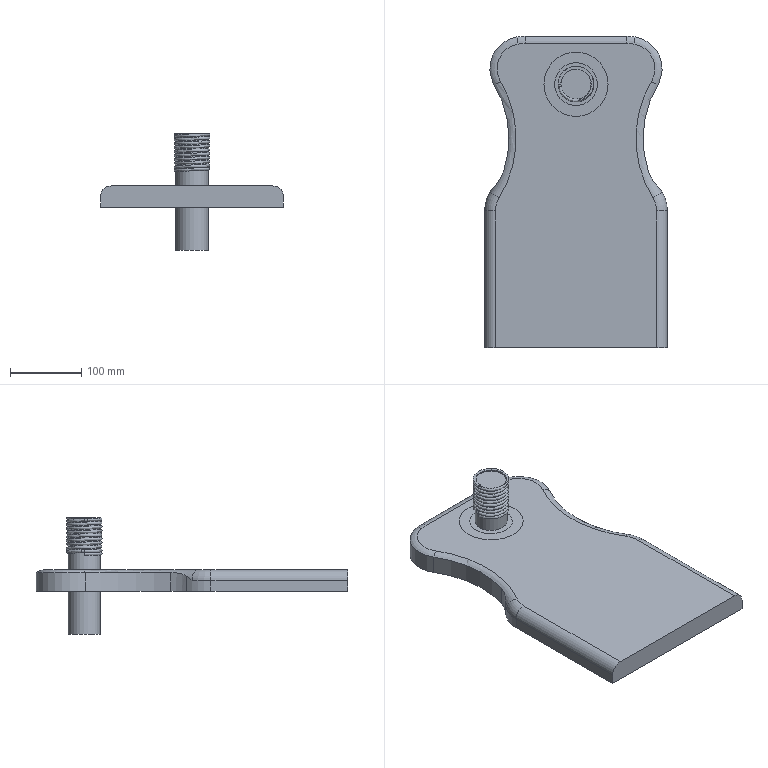Part | NX | features BREP 5 | 5 solids | 47 faces | box 256 x 436 x 165.999 mm | volume 3237071 mm3 | cylinder 19 | plane 15 | torus 8 | spline 5 | commonest cylinder face diameters 90 x4 30 x3 45 x2 60 x2 100 x2 112 x2